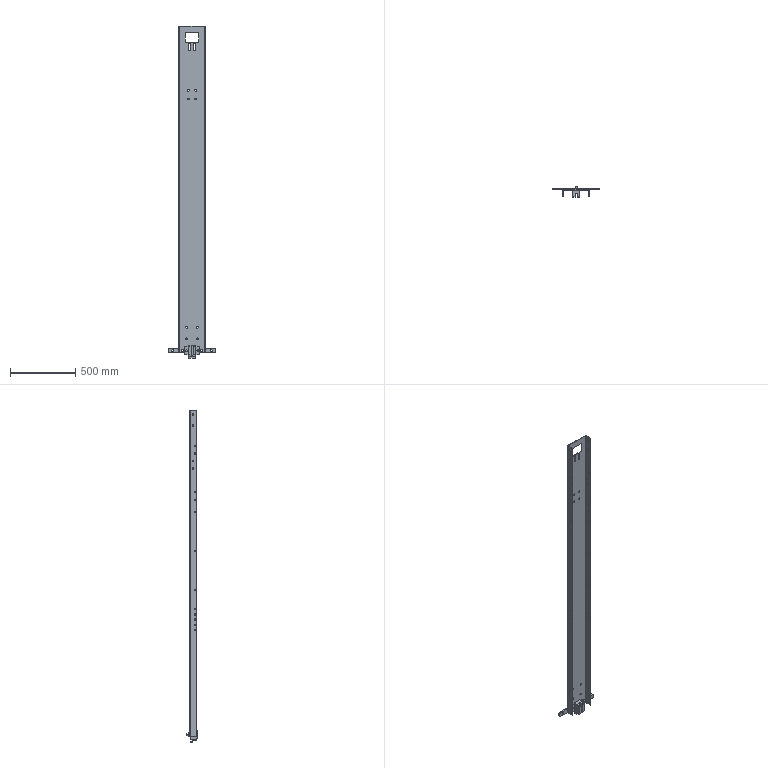Part | 4 solids | 197 faces | box 360 x 83 x 2550 mm | volume 3317757 mm3 | cylinder 116 | plane 81 | commonest cylinder face diameters 11 x40 14 x40 12.5 x8 13 x8 20 x6 12 x4